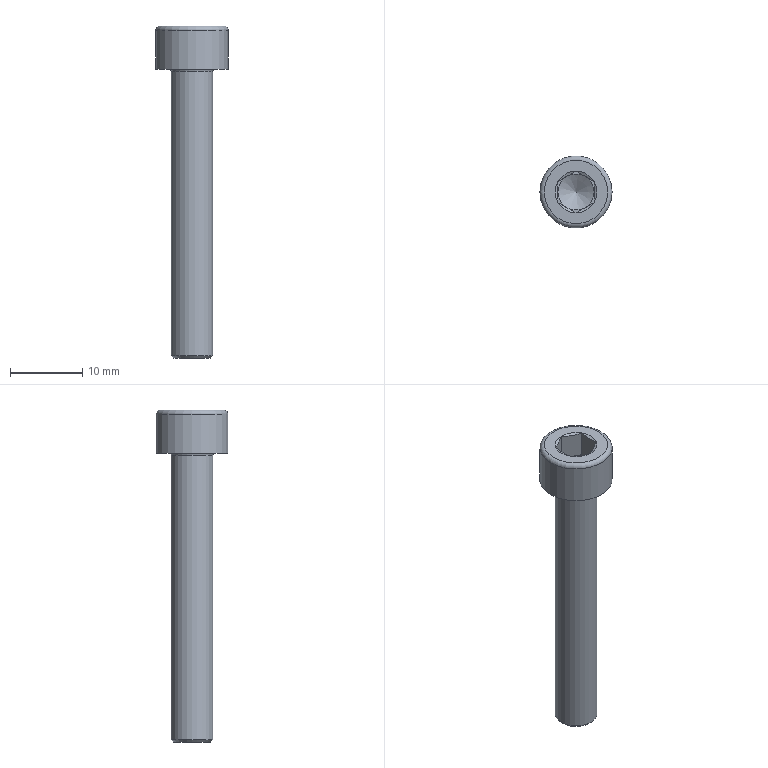Part | NX | features SKETCH 3, BLEND 2, DATUM_CSYS 2, META 2, SWP104 2, CHAMFER 1, EXTRUDE 1, LINE 1, SYMBOLIC_THREAD 1, THREADS 1 | 1 solid | 27 faces | box 10 x 10 x 46 mm | volume 1433 mm3 | plane 15 | cone 8 | cylinder 2 | torus 2 | commonest cylinder face diameters 5.795 x1 10 x1
STEP:
#1=CARTESIAN_POINT('',(-4.4,0.,6.));
#2=VERTEX_POINT('',#1);
#3=CARTESIAN_POINT('',(0.,0.,6.));
#4=DIRECTION('',(0.,0.,-1.));
#5=DIRECTION('',(-1.,0.,0.));
#6=AXIS2_PLACEMENT_3D('',#3,#4,#5);
#7=CIRCLE('',#6,4.4);
#8=EDGE_CURVE('',#2,#2,#7,.F.);
#9=ORIENTED_EDGE('',*,*,#8,.T.);
#10=EDGE_LOOP('',(#9));
#11=FACE_BOUND('',#10,.T.);
#12=CARTESIAN_POINT('',(-2.5,-1.443,6.));
#13=VERTEX_POINT('',#12);
#14=CARTESIAN_POINT('',(-2.5,1.443,6.));
#15=VERTEX_POINT('',#14);
#16=CARTESIAN_POINT('',(0.,0.,6.));
#17=DIRECTION('',(0.,0.,-1.));
#18=DIRECTION('',(-1.,0.,0.));
#19=AXIS2_PLACEMENT_3D('',#16,#17,#18);
#20=CIRCLE('',#19,2.887);
#21=EDGE_CURVE('',#13,#15,#20,.T.);
#22=ORIENTED_EDGE('',*,*,#21,.T.);
#23=CARTESIAN_POINT('',(0.,2.887,6.));
#24=VERTEX_POINT('',#23);
#25=CARTESIAN_POINT('',(0.,0.,6.));
#26=DIRECTION('',(0.,0.,-1.));
#27=DIRECTION('',(-1.,0.,0.));
#28=AXIS2_PLACEMENT_3D('',#25,#26,#27);
#29=CIRCLE('',#28,2.887);
#30=EDGE_CURVE('',#15,#24,#29,.T.);
#31=ORIENTED_EDGE('',*,*,#30,.T.);
#32=CARTESIAN_POINT('',(2.5,1.443,6.));
#33=VERTEX_POINT('',#32);
#34=CARTESIAN_POINT('',(0.,0.,6.));
#35=DIRECTION('',(0.,0.,-1.));
#36=DIRECTION('',(-1.,0.,0.));
#37=AXIS2_PLACEMENT_3D('',#34,#35,#36);
#38=CIRCLE('',#37,2.887);
#39=EDGE_CURVE('',#24,#33,#38,.T.);
#40=ORIENTED_EDGE('',*,*,#39,.T.);
#41=CARTESIAN_POINT('',(2.5,-1.443,6.));
#42=VERTEX_POINT('',#41);
#43=CARTESIAN_POINT('',(0.,0.,6.));
#44=DIRECTION('',(0.,0.,-1.));
#45=DIRECTION('',(-1.,0.,0.));
#46=AXIS2_PLACEMENT_3D('',#43,#44,#45);
#47=CIRCLE('',#46,2.887);
#48=EDGE_CURVE('',#33,#42,#47,.T.);
#49=ORIENTED_EDGE('',*,*,#48,.T.);
#50=CARTESIAN_POINT('',(0.,-2.887,6.));
#51=VERTEX_POINT('',#50);
#52=CARTESIAN_POINT('',(0.,0.,6.));
#53=DIRECTION('',(0.,0.,-1.));
#54=DIRECTION('',(-1.,0.,0.));
#55=AXIS2_PLACEMENT_3D('',#52,#53,#54);
#56=CIRCLE('',#55,2.887);
#57=EDGE_CURVE('',#42,#51,#56,.T.);
#58=ORIENTED_EDGE('',*,*,#57,.T.);
#59=CARTESIAN_POINT('',(0.,0.,6.));
#60=DIRECTION('',(0.,0.,-1.));
#61=DIRECTION('',(-1.,0.,0.));
#62=AXIS2_PLACEMENT_3D('',#59,#60,#61);
#63=CIRCLE('',#62,2.887);
#64=EDGE_CURVE('',#51,#13,#63,.T.);
#65=ORIENTED_EDGE('',*,*,#64,.T.);
#66=EDGE_LOOP('',(#22,#31,#40,#49,#58,#65));
#67=FACE_BOUND('',#66,.T.);
#68=CARTESIAN_POINT('',(0.,0.,6.));
#69=DIRECTION('',(0.,0.,-1.));
#70=DIRECTION('',(-1.,0.,0.));
#71=AXIS2_PLACEMENT_3D('',#68,#69,#70);
#72=PLANE('',#71);
#73=ADVANCED_FACE('',(#11,#67),#72,.F.);
#74=CARTESIAN_POINT('',(3.147,0.,0.));
#75=VERTEX_POINT('',#74);
#76=CARTESIAN_POINT('',(0.,0.,0.));
#77=DIRECTION('',(0.,0.,1.));
#78=DIRECTION('',(1.,0.,0.));
#79=AXIS2_PLACEMENT_3D('',#76,#77,#78);
#80=CIRCLE('',#79,3.147);
#81=EDGE_CURVE('',#75,#75,#80,.T.);
#82=ORIENTED_EDGE('',*,*,#81,.T.);
#83=EDGE_LOOP('',(#82));
#84=FACE_BOUND('',#83,.T.);
#85=CARTESIAN_POINT('',(-5.,0.,0.));
#86=VERTEX_POINT('',#85);
#87=CARTESIAN_POINT('',(0.,0.,0.));
#88=DIRECTION('',(0.,0.,-1.));
#89=DIRECTION('',(-1.,0.,0.));
#90=AXIS2_PLACEMENT_3D('',#87,#88,#89);
#91=CIRCLE('',#90,5.);
#92=EDGE_CURVE('',#86,#86,#91,.T.);
#93=ORIENTED_EDGE('',*,*,#92,.T.);
#94=EDGE_LOOP('',(#93));
#95=FACE_BOUND('',#94,.T.);
#96=CARTESIAN_POINT('',(0.,5.,0.));
#97=DIRECTION('',(0.,0.,1.));
#98=DIRECTION('',(1.,0.,0.));
#99=AXIS2_PLACEMENT_3D('',#96,#97,#98);
#100=PLANE('',#99);
#101=ADVANCED_FACE('',(#84,#95),#100,.F.);
#102=CARTESIAN_POINT('',(2.897,0.,-39.71));
#103=VERTEX_POINT('',#102);
#104=CARTESIAN_POINT('',(0.,0.,-39.71));
#105=DIRECTION('',(0.,0.,1.));
#106=DIRECTION('',(1.,0.,0.));
#107=AXIS2_PLACEMENT_3D('',#104,#105,#106);
#108=CIRCLE('',#107,2.897);
#109=EDGE_CURVE('',#103,#103,#108,.T.);
#110=ORIENTED_EDGE('',*,*,#109,.T.);
#111=EDGE_LOOP('',(#110));
#112=FACE_BOUND('',#111,.T.);
#113=CARTESIAN_POINT('',(2.897,0.,-0.25));
#114=VERTEX_POINT('',#113);
#115=CARTESIAN_POINT('',(0.,0.,-0.25));
#116=DIRECTION('',(0.,0.,1.));
#117=DIRECTION('',(1.,0.,0.));
#118=AXIS2_PLACEMENT_3D('',#115,#116,#117);
#119=CIRCLE('',#118,2.897);
#120=EDGE_CURVE('',#114,#114,#119,.F.);
#121=ORIENTED_EDGE('',*,*,#120,.T.);
#122=EDGE_LOOP('',(#121));
#123=FACE_BOUND('',#122,.T.);
#124=CARTESIAN_POINT('',(0.,0.,0.));
#125=DIRECTION('',(0.,0.,-1.));
#126=DIRECTION('',(-1.,0.,0.));
#127=AXIS2_PLACEMENT_3D('',#124,#125,#126);
#128=CYLINDRICAL_SURFACE('',#127,2.897);
#129=ADVANCED_FACE('',(#112,#123),#128,.T.);
#130=CARTESIAN_POINT('',(2.608,0.,-40.));
#131=VERTEX_POINT('',#130);
#132=CARTESIAN_POINT('',(0.,0.,-40.));
#133=DIRECTION('',(0.,0.,1.));
#134=DIRECTION('',(1.,0.,0.));
#135=AXIS2_PLACEMENT_3D('',#132,#133,#134);
#136=CIRCLE('',#135,2.608);
#137=EDGE_CURVE('',#131,#131,#136,.F.);
#138=ORIENTED_EDGE('',*,*,#137,.T.);
#139=EDGE_LOOP('',(#138));
#140=FACE_BOUND('',#139,.T.);
#141=CARTESIAN_POINT('',(0.,2.897,-40.));
#142=DIRECTION('',(0.,0.,1.));
#143=DIRECTION('',(1.,0.,0.));
#144=AXIS2_PLACEMENT_3D('',#141,#142,#143);
#145=PLANE('',#144);
#146=ADVANCED_FACE('',(#140),#145,.F.);
#147=CARTESIAN_POINT('',(-5.,0.,5.4));
#148=VERTEX_POINT('',#147);
#149=CARTESIAN_POINT('',(0.,0.,5.4));
#150=DIRECTION('',(0.,0.,-1.));
#151=DIRECTION('',(-1.,0.,0.));
#152=AXIS2_PLACEMENT_3D('',#149,#150,#151);
#153=CIRCLE('',#152,5.);
#154=EDGE_CURVE('',#148,#148,#153,.T.);
#155=ORIENTED_EDGE('',*,*,#154,.T.);
#156=EDGE_LOOP('',(#155));
#157=FACE_BOUND('',#156,.T.);
#158=ORIENTED_EDGE('',*,*,#92,.F.);
#159=EDGE_LOOP('',(#158));
#160=FACE_BOUND('',#159,.T.);
#161=CARTESIAN_POINT('',(0.,0.,0.));
#162=DIRECTION('',(0.,0.,-1.));
#163=DIRECTION('',(-1.,0.,0.));
#164=AXIS2_PLACEMENT_3D('',#161,#162,#163);
#165=CYLINDRICAL_SURFACE('',#164,5.);
#166=ADVANCED_FACE('',(#157,#160),#165,.T.);
#167=ORIENTED_EDGE('',*,*,#48,.F.);
#168=CARTESIAN_POINT('',(2.5,-1.443,6.));
#169=CARTESIAN_POINT('',(2.5,-0.5041,5.729));
#170=CARTESIAN_POINT('',(2.5,0.5101,5.731));
#171=CARTESIAN_POINT('',(2.5,1.443,6.));
#172=B_SPLINE_CURVE_WITH_KNOTS('',3,(#168,#169,#170,#171),.UNSPECIFIED.,.F.,.F.,(4,4),(0.002575,0.005496),.UNSPECIFIED.);
#173=EDGE_CURVE('',#33,#42,#172,.F.);
#174=ORIENTED_EDGE('',*,*,#173,.T.);
#175=EDGE_LOOP('',(#167,#174));
#176=FACE_BOUND('',#175,.T.);
#177=CARTESIAN_POINT('',(0.,0.,5.777));
#178=DIRECTION('',(0.,0.,1.));
#179=DIRECTION('',(1.,0.,0.));
#180=AXIS2_PLACEMENT_3D('',#177,#178,#179);
#181=CONICAL_SURFACE('',#180,2.5,1.047);
#182=ADVANCED_FACE('',(#176),#181,.F.);
#183=CARTESIAN_POINT('',(2.5,-1.443,6.));
#184=CARTESIAN_POINT('',(1.684,-1.915,5.728));
#185=CARTESIAN_POINT('',(0.8174,-2.415,5.728));
#186=CARTESIAN_POINT('',(0.,-2.887,6.));
#187=B_SPLINE_CURVE_WITH_KNOTS('',3,(#183,#184,#185,#186),.UNSPECIFIED.,.F.,.F.,(4,4),(0.000000238,0.002916),.UNSPECIFIED.);
#188=EDGE_CURVE('',#42,#51,#187,.T.);
#189=ORIENTED_EDGE('',*,*,#188,.T.);
#190=ORIENTED_EDGE('',*,*,#57,.F.);
#191=EDGE_LOOP('',(#189,#190));
#192=FACE_BOUND('',#191,.T.);
#193=CARTESIAN_POINT('',(0.,0.,5.777));
#194=DIRECTION('',(0.,0.,1.));
#195=DIRECTION('',(1.,0.,0.));
#196=AXIS2_PLACEMENT_3D('',#193,#194,#195);
#197=CONICAL_SURFACE('',#196,2.5,1.047);
#198=ADVANCED_FACE('',(#192),#197,.F.);
#199=CARTESIAN_POINT('',(0.,-2.887,6.));
#200=CARTESIAN_POINT('',(-0.8164,-2.415,5.728));
#201=CARTESIAN_POINT('',(-1.683,-1.915,5.728));
#202=CARTESIAN_POINT('',(-2.5,-1.443,6.));
#203=B_SPLINE_CURVE_WITH_KNOTS('',3,(#199,#200,#201,#202),.UNSPECIFIED.,.F.,.F.,(4,4),(0.000000238,0.002916),.UNSPECIFIED.);
#204=EDGE_CURVE('',#51,#13,#203,.T.);
#205=ORIENTED_EDGE('',*,*,#204,.T.);
#206=ORIENTED_EDGE('',*,*,#64,.F.);
#207=EDGE_LOOP('',(#205,#206));
#208=FACE_BOUND('',#207,.T.);
#209=CARTESIAN_POINT('',(0.,0.,5.777));
#210=DIRECTION('',(0.,0.,1.));
#211=DIRECTION('',(1.,0.,0.));
#212=AXIS2_PLACEMENT_3D('',#209,#210,#211);
#213=CONICAL_SURFACE('',#212,2.5,1.047);
#214=ADVANCED_FACE('',(#208),#213,.F.);
#215=CARTESIAN_POINT('',(-2.5,-1.443,6.));
#216=CARTESIAN_POINT('',(-2.5,-0.5041,5.729));
#217=CARTESIAN_POINT('',(-2.5,0.5101,5.731));
#218=CARTESIAN_POINT('',(-2.5,1.443,6.));
#219=B_SPLINE_CURVE_WITH_KNOTS('',3,(#215,#216,#217,#218),.UNSPECIFIED.,.F.,.F.,(4,4),(0.002575,0.005496),.UNSPECIFIED.);
#220=EDGE_CURVE('',#13,#15,#219,.T.);
#221=ORIENTED_EDGE('',*,*,#220,.T.);
#222=ORIENTED_EDGE('',*,*,#21,.F.);
#223=EDGE_LOOP('',(#221,#222));
#224=FACE_BOUND('',#223,.T.);
#225=CARTESIAN_POINT('',(0.,0.,5.777));
#226=DIRECTION('',(0.,0.,1.));
#227=DIRECTION('',(1.,0.,0.));
#228=AXIS2_PLACEMENT_3D('',#225,#226,#227);
#229=CONICAL_SURFACE('',#228,2.5,1.047);
#230=ADVANCED_FACE('',(#224),#229,.F.);
#231=CARTESIAN_POINT('',(-2.5,1.443,6.));
#232=CARTESIAN_POINT('',(-1.684,1.915,5.728));
#233=CARTESIAN_POINT('',(-0.8174,2.415,5.728));
#234=CARTESIAN_POINT('',(0.,2.887,6.));
#235=B_SPLINE_CURVE_WITH_KNOTS('',3,(#231,#232,#233,#234),.UNSPECIFIED.,.F.,.F.,(4,4),(0.000000238,0.002916),.UNSPECIFIED.);
#236=EDGE_CURVE('',#15,#24,#235,.T.);
#237=ORIENTED_EDGE('',*,*,#236,.T.);
#238=ORIENTED_EDGE('',*,*,#30,.F.);
#239=EDGE_LOOP('',(#237,#238));
#240=FACE_BOUND('',#239,.T.);
#241=CARTESIAN_POINT('',(0.,0.,5.777));
#242=DIRECTION('',(0.,0.,1.));
#243=DIRECTION('',(1.,0.,0.));
#244=AXIS2_PLACEMENT_3D('',#241,#242,#243);
#245=CONICAL_SURFACE('',#244,2.5,1.047);
#246=ADVANCED_FACE('',(#240),#245,.F.);
#247=CARTESIAN_POINT('',(0.,2.887,6.));
#248=CARTESIAN_POINT('',(0.8164,2.415,5.728));
#249=CARTESIAN_POINT('',(1.683,1.915,5.728));
#250=CARTESIAN_POINT('',(2.5,1.443,6.));
#251=B_SPLINE_CURVE_WITH_KNOTS('',3,(#247,#248,#249,#250),.UNSPECIFIED.,.F.,.F.,(4,4),(0.000000238,0.002916),.UNSPECIFIED.);
#252=EDGE_CURVE('',#24,#33,#251,.T.);
#253=ORIENTED_EDGE('',*,*,#252,.T.);
#254=ORIENTED_EDGE('',*,*,#39,.F.);
#255=EDGE_LOOP('',(#253,#254));
#256=FACE_BOUND('',#255,.T.);
#257=CARTESIAN_POINT('',(0.,0.,5.777));
#258=DIRECTION('',(0.,0.,1.));
#259=DIRECTION('',(1.,0.,0.));
#260=AXIS2_PLACEMENT_3D('',#257,#258,#259);
#261=CONICAL_SURFACE('',#260,2.5,1.047);
#262=ADVANCED_FACE('',(#256),#261,.F.);
#263=CARTESIAN_POINT('',(2.5,0.,2.3));
#264=VERTEX_POINT('',#263);
#265=CARTESIAN_POINT('',(1.25,2.165,2.3));
#266=VERTEX_POINT('',#265);
#267=CARTESIAN_POINT('',(0.,0.,2.3));
#268=DIRECTION('',(0.,0.,1.));
#269=DIRECTION('',(1.,0.,0.));
#270=AXIS2_PLACEMENT_3D('',#267,#268,#269);
#271=CIRCLE('',#270,2.5);
#272=EDGE_CURVE('',#264,#266,#271,.T.);
#273=ORIENTED_EDGE('',*,*,#272,.F.);
#274=CARTESIAN_POINT('',(2.5,1.443,2.3));
#275=VERTEX_POINT('',#274);
#276=CARTESIAN_POINT('',(2.5,-1.443,2.3));
#277=DIRECTION('',(0.,1.,0.));
#278=VECTOR('',#277,1000.);
#279=LINE('',#276,#278);
#280=EDGE_CURVE('',#264,#275,#279,.T.);
#281=ORIENTED_EDGE('',*,*,#280,.T.);
#282=CARTESIAN_POINT('',(2.5,1.443,2.3));
#283=DIRECTION('',(-0.866,0.5,0.));
#284=VECTOR('',#283,1000.);
#285=LINE('',#282,#284);
#286=EDGE_CURVE('',#275,#266,#285,.T.);
#287=ORIENTED_EDGE('',*,*,#286,.T.);
#288=EDGE_LOOP('',(#273,#281,#287));
#289=FACE_BOUND('',#288,.T.);
#290=CARTESIAN_POINT('',(-2.5,4.33,2.3));
#291=DIRECTION('',(0.,0.,1.));
#292=DIRECTION('',(1.,0.,0.));
#293=AXIS2_PLACEMENT_3D('',#290,#291,#292);
#294=PLANE('',#293);
#295=ADVANCED_FACE('',(#289),#294,.T.);
#296=CARTESIAN_POINT('',(1.25,-2.165,2.3));
#297=VERTEX_POINT('',#296);
#298=CARTESIAN_POINT('',(0.,0.,2.3));
#299=DIRECTION('',(0.,0.,1.));
#300=DIRECTION('',(1.,0.,0.));
#301=AXIS2_PLACEMENT_3D('',#298,#299,#300);
#302=CIRCLE('',#301,2.5);
#303=EDGE_CURVE('',#297,#264,#302,.T.);
#304=ORIENTED_EDGE('',*,*,#303,.F.);
#305=CARTESIAN_POINT('',(2.5,-1.443,2.3));
#306=VERTEX_POINT('',#305);
#307=CARTESIAN_POINT('',(0.,-2.887,2.3));
#308=DIRECTION('',(0.866,0.5,0.));
#309=VECTOR('',#308,1000.);
#310=LINE('',#307,#309);
#311=EDGE_CURVE('',#297,#306,#310,.T.);
#312=ORIENTED_EDGE('',*,*,#311,.T.);
#313=CARTESIAN_POINT('',(2.5,-1.443,2.3));
#314=DIRECTION('',(0.,1.,0.));
#315=VECTOR('',#314,1000.);
#316=LINE('',#313,#315);
#317=EDGE_CURVE('',#306,#264,#316,.T.);
#318=ORIENTED_EDGE('',*,*,#317,.T.);
#319=EDGE_LOOP('',(#304,#312,#318));
#320=FACE_BOUND('',#319,.T.);
#321=CARTESIAN_POINT('',(-2.5,4.33,2.3));
#322=DIRECTION('',(0.,0.,1.));
#323=DIRECTION('',(1.,0.,0.));
#324=AXIS2_PLACEMENT_3D('',#321,#322,#323);
#325=PLANE('',#324);
#326=ADVANCED_FACE('',(#320),#325,.T.);
#327=ORIENTED_EDGE('',*,*,#280,.F.);
#328=ORIENTED_EDGE('',*,*,#317,.F.);
#329=CARTESIAN_POINT('',(2.5,-1.443,6.));
#330=DIRECTION('',(0.,0.,-1.));
#331=VECTOR('',#330,1000.);
#332=LINE('',#329,#331);
#333=EDGE_CURVE('',#42,#306,#332,.T.);
#334=ORIENTED_EDGE('',*,*,#333,.F.);
#335=ORIENTED_EDGE('',*,*,#173,.F.);
#336=CARTESIAN_POINT('',(2.5,1.443,6.));
#337=DIRECTION('',(0.,0.,-1.));
#338=VECTOR('',#337,1000.);
#339=LINE('',#336,#338);
#340=EDGE_CURVE('',#33,#275,#339,.T.);
#341=ORIENTED_EDGE('',*,*,#340,.T.);
#342=EDGE_LOOP('',(#327,#328,#334,#335,#341));
#343=FACE_BOUND('',#342,.T.);
#344=CARTESIAN_POINT('',(2.5,-1.443,6.));
#345=DIRECTION('',(-1.,0.,0.));
#346=DIRECTION('',(0.,0.,1.));
#347=AXIS2_PLACEMENT_3D('',#344,#345,#346);
#348=PLANE('',#347);
#349=ADVANCED_FACE('',(#343),#348,.T.);
#350=CARTESIAN_POINT('',(-1.25,-2.165,2.3));
#351=VERTEX_POINT('',#350);
#352=CARTESIAN_POINT('',(0.,0.,2.3));
#353=DIRECTION('',(0.,0.,1.));
#354=DIRECTION('',(1.,0.,0.));
#355=AXIS2_PLACEMENT_3D('',#352,#353,#354);
#356=CIRCLE('',#355,2.5);
#357=EDGE_CURVE('',#351,#297,#356,.T.);
#358=ORIENTED_EDGE('',*,*,#357,.F.);
#359=CARTESIAN_POINT('',(0.,-2.887,2.3));
#360=VERTEX_POINT('',#359);
#361=CARTESIAN_POINT('',(-2.5,-1.443,2.3));
#362=DIRECTION('',(0.866,-0.5,0.));
#363=VECTOR('',#362,1000.);
#364=LINE('',#361,#363);
#365=EDGE_CURVE('',#351,#360,#364,.T.);
#366=ORIENTED_EDGE('',*,*,#365,.T.);
#367=CARTESIAN_POINT('',(0.,-2.887,2.3));
#368=DIRECTION('',(0.866,0.5,0.));
#369=VECTOR('',#368,1000.);
#370=LINE('',#367,#369);
#371=EDGE_CURVE('',#360,#297,#370,.T.);
#372=ORIENTED_EDGE('',*,*,#371,.T.);
#373=EDGE_LOOP('',(#358,#366,#372));
#374=FACE_BOUND('',#373,.T.);
#375=CARTESIAN_POINT('',(-2.5,4.33,2.3));
#376=DIRECTION('',(0.,0.,1.));
#377=DIRECTION('',(1.,0.,0.));
#378=AXIS2_PLACEMENT_3D('',#375,#376,#377);
#379=PLANE('',#378);
#380=ADVANCED_FACE('',(#374),#379,.T.);
#381=ORIENTED_EDGE('',*,*,#311,.F.);
#382=ORIENTED_EDGE('',*,*,#371,.F.);
#383=CARTESIAN_POINT('',(0.,-2.887,6.));
#384=DIRECTION('',(0.,0.,-1.));
#385=VECTOR('',#384,1000.);
#386=LINE('',#383,#385);
#387=EDGE_CURVE('',#51,#360,#386,.T.);
#388=ORIENTED_EDGE('',*,*,#387,.F.);
#389=ORIENTED_EDGE('',*,*,#188,.F.);
#390=ORIENTED_EDGE('',*,*,#333,.T.);
#391=EDGE_LOOP('',(#381,#382,#388,#389,#390));
#392=FACE_BOUND('',#391,.T.);
#393=CARTESIAN_POINT('',(0.,-2.887,6.));
#394=DIRECTION('',(-0.5,0.866,0.));
#395=DIRECTION('',(-0.866,-0.5,0.));
#396=AXIS2_PLACEMENT_3D('',#393,#394,#395);
#397=PLANE('',#396);
#398=ADVANCED_FACE('',(#392),#397,.T.);
#399=CARTESIAN_POINT('',(-2.5,0.,2.3));
#400=VERTEX_POINT('',#399);
#401=CARTESIAN_POINT('',(0.,0.,2.3));
#402=DIRECTION('',(0.,0.,1.));
#403=DIRECTION('',(1.,0.,0.));
#404=AXIS2_PLACEMENT_3D('',#401,#402,#403);
#405=CIRCLE('',#404,2.5);
#406=EDGE_CURVE('',#400,#351,#405,.T.);
#407=ORIENTED_EDGE('',*,*,#406,.F.);
#408=CARTESIAN_POINT('',(-2.5,-1.443,2.3));
#409=VERTEX_POINT('',#408);
#410=CARTESIAN_POINT('',(-2.5,1.443,2.3));
#411=DIRECTION('',(0.,-1.,0.));
#412=VECTOR('',#411,1000.);
#413=LINE('',#410,#412);
#414=EDGE_CURVE('',#400,#409,#413,.T.);
#415=ORIENTED_EDGE('',*,*,#414,.T.);
#416=CARTESIAN_POINT('',(-2.5,-1.443,2.3));
#417=DIRECTION('',(0.866,-0.5,0.));
#418=VECTOR('',#417,1000.);
#419=LINE('',#416,#418);
#420=EDGE_CURVE('',#409,#351,#419,.T.);
#421=ORIENTED_EDGE('',*,*,#420,.T.);
#422=EDGE_LOOP('',(#407,#415,#421));
#423=FACE_BOUND('',#422,.T.);
#424=CARTESIAN_POINT('',(-2.5,4.33,2.3));
#425=DIRECTION('',(0.,0.,1.));
#426=DIRECTION('',(1.,0.,0.));
#427=AXIS2_PLACEMENT_3D('',#424,#425,#426);
#428=PLANE('',#427);
#429=ADVANCED_FACE('',(#423),#428,.T.);
#430=ORIENTED_EDGE('',*,*,#365,.F.);
#431=ORIENTED_EDGE('',*,*,#420,.F.);
#432=CARTESIAN_POINT('',(-2.5,-1.443,6.));
#433=DIRECTION('',(0.,0.,-1.));
#434=VECTOR('',#433,1000.);
#435=LINE('',#432,#434);
#436=EDGE_CURVE('',#13,#409,#435,.T.);
#437=ORIENTED_EDGE('',*,*,#436,.F.);
#438=ORIENTED_EDGE('',*,*,#204,.F.);
#439=ORIENTED_EDGE('',*,*,#387,.T.);
#440=EDGE_LOOP('',(#430,#431,#437,#438,#439));
#441=FACE_BOUND('',#440,.T.);
#442=CARTESIAN_POINT('',(-2.5,-1.443,6.));
#443=DIRECTION('',(0.5,0.866,0.));
#444=DIRECTION('',(-0.866,0.5,0.));
#445=AXIS2_PLACEMENT_3D('',#442,#443,#444);
#446=PLANE('',#445);
#447=ADVANCED_FACE('',(#441),#446,.T.);
#448=CARTESIAN_POINT('',(-1.25,2.165,2.3));
#449=VERTEX_POINT('',#448);
#450=CARTESIAN_POINT('',(0.,0.,2.3));
#451=DIRECTION('',(0.,0.,-1.));
#452=DIRECTION('',(-1.,0.,0.));
#453=AXIS2_PLACEMENT_3D('',#450,#451,#452);
#454=CIRCLE('',#453,2.5);
#455=EDGE_CURVE('',#400,#449,#454,.T.);
#456=ORIENTED_EDGE('',*,*,#455,.T.);
#457=CARTESIAN_POINT('',(-2.5,1.443,2.3));
#458=VERTEX_POINT('',#457);
#459=CARTESIAN_POINT('',(0.,2.887,2.3));
#460=DIRECTION('',(-0.866,-0.5,0.));
#461=VECTOR('',#460,1000.);
#462=LINE('',#459,#461);
#463=EDGE_CURVE('',#449,#458,#462,.T.);
#464=ORIENTED_EDGE('',*,*,#463,.T.);
#465=CARTESIAN_POINT('',(-2.5,1.443,2.3));
#466=DIRECTION('',(0.,-1.,0.));
#467=VECTOR('',#466,1000.);
#468=LINE('',#465,#467);
#469=EDGE_CURVE('',#458,#400,#468,.T.);
#470=ORIENTED_EDGE('',*,*,#469,.T.);
#471=EDGE_LOOP('',(#456,#464,#470));
#472=FACE_BOUND('',#471,.T.);
#473=CARTESIAN_POINT('',(-2.5,4.33,2.3));
#474=DIRECTION('',(0.,0.,1.));
#475=DIRECTION('',(1.,0.,0.));
#476=AXIS2_PLACEMENT_3D('',#473,#474,#475);
#477=PLANE('',#476);
#478=ADVANCED_FACE('',(#472),#477,.T.);
#479=ORIENTED_EDGE('',*,*,#414,.F.);
#480=ORIENTED_EDGE('',*,*,#469,.F.);
#481=CARTESIAN_POINT('',(-2.5,1.443,6.));
#482=DIRECTION('',(0.,0.,-1.));
#483=VECTOR('',#482,1000.);
#484=LINE('',#481,#483);
#485=EDGE_CURVE('',#15,#458,#484,.T.);
#486=ORIENTED_EDGE('',*,*,#485,.F.);
#487=ORIENTED_EDGE('',*,*,#220,.F.);
#488=ORIENTED_EDGE('',*,*,#436,.T.);
#489=EDGE_LOOP('',(#479,#480,#486,#487,#488));
#490=FACE_BOUND('',#489,.T.);
#491=CARTESIAN_POINT('',(-2.5,1.443,6.));
#492=DIRECTION('',(1.,0.,0.));
#493=DIRECTION('',(0.,0.,-1.));
#494=AXIS2_PLACEMENT_3D('',#491,#492,#493);
#495=PLANE('',#494);
#496=ADVANCED_FACE('',(#490),#495,.T.);
#497=CARTESIAN_POINT('',(0.,0.,2.3));
#498=DIRECTION('',(0.,0.,1.));
#499=DIRECTION('',(1.,0.,0.));
#500=AXIS2_PLACEMENT_3D('',#497,#498,#499);
#501=CIRCLE('',#500,2.5);
#502=EDGE_CURVE('',#266,#449,#501,.T.);
#503=ORIENTED_EDGE('',*,*,#502,.F.);
#504=CARTESIAN_POINT('',(0.,2.887,2.3));
#505=VERTEX_POINT('',#504);
#506=CARTESIAN_POINT('',(2.5,1.443,2.3));
#507=DIRECTION('',(-0.866,0.5,0.));
#508=VECTOR('',#507,1000.);
#509=LINE('',#506,#508);
#510=EDGE_CURVE('',#266,#505,#509,.T.);
#511=ORIENTED_EDGE('',*,*,#510,.T.);
#512=CARTESIAN_POINT('',(0.,2.887,2.3));
#513=DIRECTION('',(-0.866,-0.5,0.));
#514=VECTOR('',#513,1000.);
#515=LINE('',#512,#514);
#516=EDGE_CURVE('',#505,#449,#515,.T.);
#517=ORIENTED_EDGE('',*,*,#516,.T.);
#518=EDGE_LOOP('',(#503,#511,#517));
#519=FACE_BOUND('',#518,.T.);
#520=CARTESIAN_POINT('',(-2.5,4.33,2.3));
#521=DIRECTION('',(0.,0.,1.));
#522=DIRECTION('',(1.,0.,0.));
#523=AXIS2_PLACEMENT_3D('',#520,#521,#522);
#524=PLANE('',#523);
#525=ADVANCED_FACE('',(#519),#524,.T.);
#526=ORIENTED_EDGE('',*,*,#463,.F.);
#527=ORIENTED_EDGE('',*,*,#516,.F.);
#528=CARTESIAN_POINT('',(0.,2.887,6.));
#529=DIRECTION('',(0.,0.,-1.));
#530=VECTOR('',#529,1000.);
#531=LINE('',#528,#530);
#532=EDGE_CURVE('',#24,#505,#531,.T.);
#533=ORIENTED_EDGE('',*,*,#532,.F.);
#534=ORIENTED_EDGE('',*,*,#236,.F.);
#535=ORIENTED_EDGE('',*,*,#485,.T.);
#536=EDGE_LOOP('',(#526,#527,#533,#534,#535));
#537=FACE_BOUND('',#536,.T.);
#538=CARTESIAN_POINT('',(0.,2.887,6.));
#539=DIRECTION('',(0.5,-0.866,0.));
#540=DIRECTION('',(0.866,0.5,0.));
#541=AXIS2_PLACEMENT_3D('',#538,#539,#540);
#542=PLANE('',#541);
#543=ADVANCED_FACE('',(#537),#542,.T.);
#544=ORIENTED_EDGE('',*,*,#510,.F.);
#545=ORIENTED_EDGE('',*,*,#286,.F.);
#546=ORIENTED_EDGE('',*,*,#340,.F.);
#547=ORIENTED_EDGE('',*,*,#252,.F.);
#548=ORIENTED_EDGE('',*,*,#532,.T.);
#549=EDGE_LOOP('',(#544,#545,#546,#547,#548));
#550=FACE_BOUND('',#549,.T.);
#551=CARTESIAN_POINT('',(2.5,1.443,6.));
#552=DIRECTION('',(-0.5,-0.866,0.));
#553=DIRECTION('',(0.866,-0.5,0.));
#554=AXIS2_PLACEMENT_3D('',#551,#552,#553);
#555=PLANE('',#554);
#556=ADVANCED_FACE('',(#550),#555,.T.);
#557=ORIENTED_EDGE('',*,*,#455,.F.);
#558=ORIENTED_EDGE('',*,*,#406,.T.);
#559=ORIENTED_EDGE('',*,*,#357,.T.);
#560=ORIENTED_EDGE('',*,*,#303,.T.);
#561=ORIENTED_EDGE('',*,*,#272,.T.);
#562=ORIENTED_EDGE('',*,*,#502,.T.);
#563=EDGE_LOOP('',(#557,#558,#559,#560,#561,#562));
#564=FACE_BOUND('',#563,.T.);
#565=CARTESIAN_POINT('',(0.,0.,0.8566));
#566=VERTEX_POINT('',#565);
#567=VERTEX_LOOP('',#566);
#568=FACE_BOUND('',#567,.T.);
#569=CARTESIAN_POINT('',(0.,0.,0.8566));
#570=DIRECTION('',(0.,0.,1.));
#571=DIRECTION('',(1.,0.,0.));
#572=AXIS2_PLACEMENT_3D('',#569,#570,#571);
#573=CONICAL_SURFACE('',#572,0.,1.047);
#574=ADVANCED_FACE('',(#564,#568),#573,.F.);
#575=ORIENTED_EDGE('',*,*,#8,.F.);
#576=EDGE_LOOP('',(#575));
#577=FACE_BOUND('',#576,.T.);
#578=ORIENTED_EDGE('',*,*,#154,.F.);
#579=EDGE_LOOP('',(#578));
#580=FACE_BOUND('',#579,.T.);
#581=CARTESIAN_POINT('',(0.,0.,5.4));
#582=DIRECTION('',(0.,0.,-1.));
#583=DIRECTION('',(-1.,0.,0.));
#584=AXIS2_PLACEMENT_3D('',#581,#582,#583);
#585=TOROIDAL_SURFACE('',#584,4.4,0.6);
#586=ADVANCED_FACE('',(#577,#580),#585,.T.);
#587=ORIENTED_EDGE('',*,*,#81,.F.);
#588=EDGE_LOOP('',(#587));
#589=FACE_BOUND('',#588,.T.);
#590=ORIENTED_EDGE('',*,*,#120,.F.);
#591=EDGE_LOOP('',(#590));
#592=FACE_BOUND('',#591,.T.);
#593=CARTESIAN_POINT('',(0.,0.,-0.25));
#594=DIRECTION('',(0.,0.,1.));
#595=DIRECTION('',(1.,0.,0.));
#596=AXIS2_PLACEMENT_3D('',#593,#594,#595);
#597=TOROIDAL_SURFACE('',#596,3.147,0.25);
#598=ADVANCED_FACE('',(#589,#592),#597,.F.);
#599=ORIENTED_EDGE('',*,*,#109,.F.);
#600=EDGE_LOOP('',(#599));
#601=FACE_BOUND('',#600,.T.);
#602=ORIENTED_EDGE('',*,*,#137,.F.);
#603=EDGE_LOOP('',(#602));
#604=FACE_BOUND('',#603,.T.);
#605=CARTESIAN_POINT('',(0.,0.,-40.));
#606=DIRECTION('',(0.,0.,1.));
#607=DIRECTION('',(1.,0.,0.));
#608=AXIS2_PLACEMENT_3D('',#605,#606,#607);
#609=CONICAL_SURFACE('',#608,2.608,0.7854);
#610=ADVANCED_FACE('',(#601,#604),#609,.T.);
#611=CLOSED_SHELL('',(#73,#101,#129,#146,#166,#182,#198,#214,#230,#246,#262,#295,#326,#349,#380,#398,#429,#447,#478,#496,#525,#543,#556,#574,#586,#598,#610));
#612=MANIFOLD_SOLID_BREP('',#611);
#613=(LENGTH_UNIT()NAMED_UNIT(*)SI_UNIT(.MILLI.,.METRE.));
#614=UNCERTAINTY_MEASURE_WITH_UNIT(LENGTH_MEASURE(0.0508),#613,'','');
#615=(NAMED_UNIT(*)PLANE_ANGLE_UNIT()SI_UNIT($,.RADIAN.));
#616=(NAMED_UNIT(*)SI_UNIT($,.STERADIAN.)SOLID_ANGLE_UNIT());
#617=(GEOMETRIC_REPRESENTATION_CONTEXT(3)GLOBAL_UNCERTAINTY_ASSIGNED_CONTEXT((#614))GLOBAL_UNIT_ASSIGNED_CONTEXT((#613,#615,#616))REPRESENTATION_CONTEXT('',''));
#618=ADVANCED_BREP_SHAPE_REPRESENTATION('',(#612),#617);